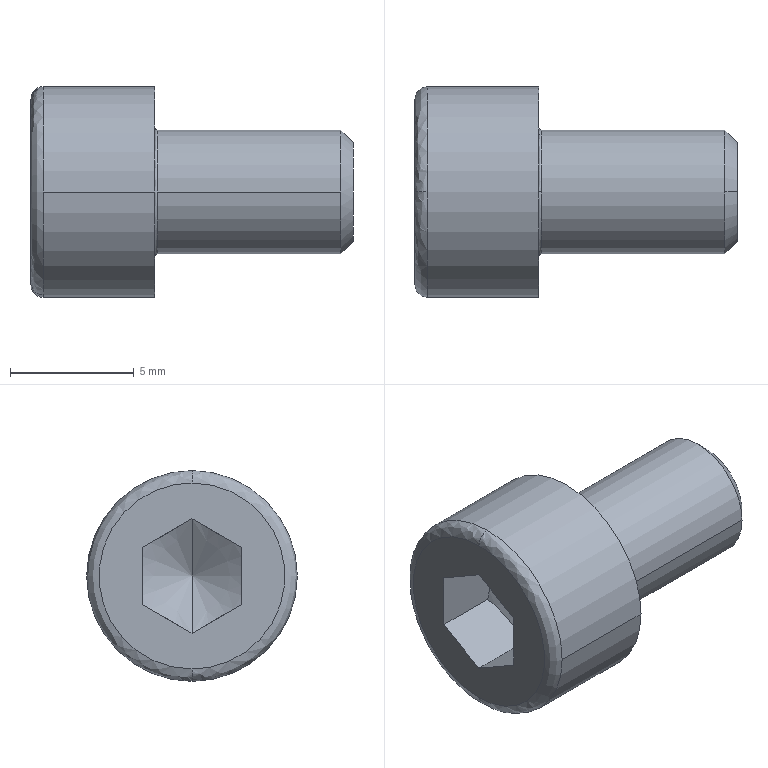Part | STEP file | DIN 912 - replaced by DIN EN ISO 4762 M5 x 8 | 1 solid | 21 faces | box 13 x 8.5 x 8.5 mm | volume 395.808 mm3 | plane 9 | spline 4 | cylinder 4 | cone 4 | commonest cylinder face diameters 5 x2 8.5 x2